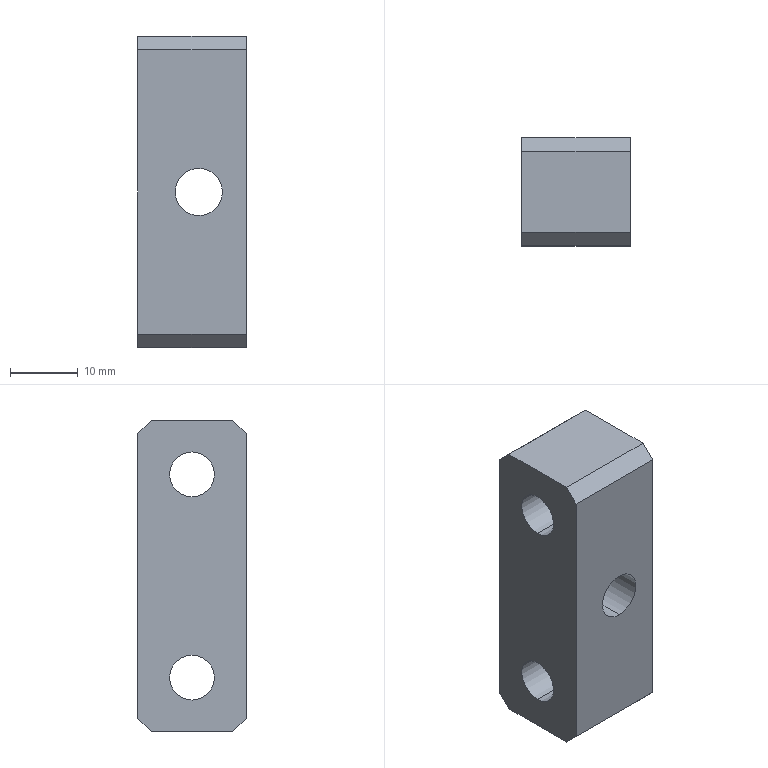Part | SolidWorks | features BaseBody 1 | 1 solid | 22 faces | box 16 x 16 x 46 mm | volume 9089 mm3 | plane 12 | cylinder 10 | commonest cylinder face diameters 6.6 x4 11 x4 6.985 x2
STEP:
#1=CARTESIAN_POINT('',(7.,0.,-20.5));
#2=VERTEX_POINT('',#1);
#3=CARTESIAN_POINT('',(7.,0.,-9.5));
#4=VERTEX_POINT('',#3);
#5=CARTESIAN_POINT('',(7.,0.,-15.));
#6=DIRECTION('',(1.,0.,0.));
#7=DIRECTION('',(0.,0.,-1.));
#8=AXIS2_PLACEMENT_3D('',#5,#6,#7);
#9=CIRCLE('',#8,5.5);
#10=EDGE_CURVE('',#2,#4,#9,.T.);
#11=ORIENTED_EDGE('',*,*,#10,.T.);
#12=CARTESIAN_POINT('',(0.,0.,-9.5));
#13=VERTEX_POINT('',#12);
#14=CARTESIAN_POINT('',(9.,0.,-9.5));
#15=DIRECTION('',(-1.,0.,0.));
#16=VECTOR('',#15,1000.);
#17=LINE('',#14,#16);
#18=EDGE_CURVE('',#4,#13,#17,.T.);
#19=ORIENTED_EDGE('',*,*,#18,.T.);
#20=CARTESIAN_POINT('',(0.,0.,-20.5));
#21=VERTEX_POINT('',#20);
#22=CARTESIAN_POINT('',(0.,0.,-15.));
#23=DIRECTION('',(1.,0.,0.));
#24=DIRECTION('',(0.,0.,-1.));
#25=AXIS2_PLACEMENT_3D('',#22,#23,#24);
#26=CIRCLE('',#25,5.5);
#27=EDGE_CURVE('',#21,#13,#26,.T.);
#28=ORIENTED_EDGE('',*,*,#27,.F.);
#29=CARTESIAN_POINT('',(9.,0.,-20.5));
#30=DIRECTION('',(-1.,0.,0.));
#31=VECTOR('',#30,1000.);
#32=LINE('',#29,#31);
#33=EDGE_CURVE('',#2,#21,#32,.T.);
#34=ORIENTED_EDGE('',*,*,#33,.F.);
#35=EDGE_LOOP('',(#11,#19,#28,#34));
#36=FACE_OUTER_BOUND('',#35,.T.);
#37=CARTESIAN_POINT('',(9.,0.,-15.));
#38=DIRECTION('',(-1.,0.,0.));
#39=DIRECTION('',(0.,0.,-1.));
#40=AXIS2_PLACEMENT_3D('',#37,#38,#39);
#41=CYLINDRICAL_SURFACE('',#40,5.5);
#42=ADVANCED_FACE('',(#36),#41,.F.);
#43=CARTESIAN_POINT('',(0.,0.,-18.3));
#44=VERTEX_POINT('',#43);
#45=CARTESIAN_POINT('',(0.,0.,-11.7));
#46=VERTEX_POINT('',#45);
#47=CARTESIAN_POINT('',(0.,0.,-15.));
#48=DIRECTION('',(1.,0.,0.));
#49=DIRECTION('',(0.,0.,-1.));
#50=AXIS2_PLACEMENT_3D('',#47,#48,#49);
#51=CIRCLE('',#50,3.3);
#52=EDGE_CURVE('',#44,#46,#51,.T.);
#53=ORIENTED_EDGE('',*,*,#52,.T.);
#54=CARTESIAN_POINT('',(-9.,0.,-11.7));
#55=VERTEX_POINT('',#54);
#56=CARTESIAN_POINT('',(-41.,0.,-11.7));
#57=DIRECTION('',(-1.,0.,0.));
#58=VECTOR('',#57,1000.);
#59=LINE('',#56,#58);
#60=EDGE_CURVE('',#46,#55,#59,.T.);
#61=ORIENTED_EDGE('',*,*,#60,.T.);
#62=CARTESIAN_POINT('',(-9.,0.,-18.3));
#63=VERTEX_POINT('',#62);
#64=CARTESIAN_POINT('',(-9.,0.,-15.));
#65=DIRECTION('',(1.,0.,0.));
#66=DIRECTION('',(0.,0.,-1.));
#67=AXIS2_PLACEMENT_3D('',#64,#65,#66);
#68=CIRCLE('',#67,3.3);
#69=EDGE_CURVE('',#63,#55,#68,.T.);
#70=ORIENTED_EDGE('',*,*,#69,.F.);
#71=CARTESIAN_POINT('',(-41.,0.,-18.3));
#72=DIRECTION('',(-1.,0.,0.));
#73=VECTOR('',#72,1000.);
#74=LINE('',#71,#73);
#75=EDGE_CURVE('',#44,#63,#74,.T.);
#76=ORIENTED_EDGE('',*,*,#75,.F.);
#77=EDGE_LOOP('',(#53,#61,#70,#76));
#78=FACE_OUTER_BOUND('',#77,.T.);
#79=CARTESIAN_POINT('',(-41.,0.,-15.));
#80=DIRECTION('',(-1.,0.,0.));
#81=DIRECTION('',(0.,0.,-1.));
#82=AXIS2_PLACEMENT_3D('',#79,#80,#81);
#83=CYLINDRICAL_SURFACE('',#82,3.3);
#84=ADVANCED_FACE('',(#78),#83,.F.);
#85=CARTESIAN_POINT('',(7.,0.,9.5));
#86=VERTEX_POINT('',#85);
#87=CARTESIAN_POINT('',(7.,0.,20.5));
#88=VERTEX_POINT('',#87);
#89=CARTESIAN_POINT('',(7.,0.,15.));
#90=DIRECTION('',(-1.,0.,0.));
#91=DIRECTION('',(0.,0.,1.));
#92=AXIS2_PLACEMENT_3D('',#89,#90,#91);
#93=CIRCLE('',#92,5.5);
#94=EDGE_CURVE('',#86,#88,#93,.T.);
#95=ORIENTED_EDGE('',*,*,#94,.F.);
#96=CARTESIAN_POINT('',(0.,0.,9.5));
#97=VERTEX_POINT('',#96);
#98=CARTESIAN_POINT('',(9.,0.,9.5));
#99=DIRECTION('',(-1.,0.,0.));
#100=VECTOR('',#99,1000.);
#101=LINE('',#98,#100);
#102=EDGE_CURVE('',#86,#97,#101,.T.);
#103=ORIENTED_EDGE('',*,*,#102,.T.);
#104=CARTESIAN_POINT('',(0.,0.,20.5));
#105=VERTEX_POINT('',#104);
#106=CARTESIAN_POINT('',(0.,0.,15.));
#107=DIRECTION('',(-1.,0.,0.));
#108=DIRECTION('',(0.,0.,1.));
#109=AXIS2_PLACEMENT_3D('',#106,#107,#108);
#110=CIRCLE('',#109,5.5);
#111=EDGE_CURVE('',#97,#105,#110,.T.);
#112=ORIENTED_EDGE('',*,*,#111,.T.);
#113=CARTESIAN_POINT('',(9.,0.,20.5));
#114=DIRECTION('',(-1.,0.,0.));
#115=VECTOR('',#114,1000.);
#116=LINE('',#113,#115);
#117=EDGE_CURVE('',#88,#105,#116,.T.);
#118=ORIENTED_EDGE('',*,*,#117,.F.);
#119=EDGE_LOOP('',(#95,#103,#112,#118));
#120=FACE_OUTER_BOUND('',#119,.T.);
#121=CARTESIAN_POINT('',(9.,0.,15.));
#122=DIRECTION('',(-1.,0.,0.));
#123=DIRECTION('',(0.,0.,1.));
#124=AXIS2_PLACEMENT_3D('',#121,#122,#123);
#125=CYLINDRICAL_SURFACE('',#124,5.5);
#126=ADVANCED_FACE('',(#120),#125,.F.);
#127=CARTESIAN_POINT('',(0.,0.,11.7));
#128=VERTEX_POINT('',#127);
#129=CARTESIAN_POINT('',(0.,0.,18.3));
#130=VERTEX_POINT('',#129);
#131=CARTESIAN_POINT('',(0.,0.,15.));
#132=DIRECTION('',(-1.,0.,0.));
#133=DIRECTION('',(0.,0.,1.));
#134=AXIS2_PLACEMENT_3D('',#131,#132,#133);
#135=CIRCLE('',#134,3.3);
#136=EDGE_CURVE('',#128,#130,#135,.T.);
#137=ORIENTED_EDGE('',*,*,#136,.F.);
#138=CARTESIAN_POINT('',(-9.,0.,11.7));
#139=VERTEX_POINT('',#138);
#140=CARTESIAN_POINT('',(-41.,0.,11.7));
#141=DIRECTION('',(-1.,0.,0.));
#142=VECTOR('',#141,1000.);
#143=LINE('',#140,#142);
#144=EDGE_CURVE('',#128,#139,#143,.T.);
#145=ORIENTED_EDGE('',*,*,#144,.T.);
#146=CARTESIAN_POINT('',(-9.,0.,18.3));
#147=VERTEX_POINT('',#146);
#148=CARTESIAN_POINT('',(-9.,0.,15.));
#149=DIRECTION('',(1.,0.,0.));
#150=DIRECTION('',(0.,0.,-1.));
#151=AXIS2_PLACEMENT_3D('',#148,#149,#150);
#152=CIRCLE('',#151,3.3);
#153=EDGE_CURVE('',#147,#139,#152,.T.);
#154=ORIENTED_EDGE('',*,*,#153,.F.);
#155=CARTESIAN_POINT('',(-41.,0.,18.3));
#156=DIRECTION('',(-1.,0.,0.));
#157=VECTOR('',#156,1000.);
#158=LINE('',#155,#157);
#159=EDGE_CURVE('',#130,#147,#158,.T.);
#160=ORIENTED_EDGE('',*,*,#159,.F.);
#161=EDGE_LOOP('',(#137,#145,#154,#160));
#162=FACE_OUTER_BOUND('',#161,.T.);
#163=CARTESIAN_POINT('',(-41.,0.,15.));
#164=DIRECTION('',(-1.,0.,0.));
#165=DIRECTION('',(0.,0.,1.));
#166=AXIS2_PLACEMENT_3D('',#163,#164,#165);
#167=CYLINDRICAL_SURFACE('',#166,3.3);
#168=ADVANCED_FACE('',(#162),#167,.F.);
#169=CARTESIAN_POINT('',(0.,-8.,-3.493));
#170=VERTEX_POINT('',#169);
#171=CARTESIAN_POINT('',(0.,-8.,3.493));
#172=VERTEX_POINT('',#171);
#173=CARTESIAN_POINT('',(0.,-8.,0.));
#174=DIRECTION('',(0.,1.,0.));
#175=DIRECTION('',(0.,0.,1.));
#176=AXIS2_PLACEMENT_3D('',#173,#174,#175);
#177=CIRCLE('',#176,3.493);
#178=EDGE_CURVE('',#170,#172,#177,.T.);
#179=ORIENTED_EDGE('',*,*,#178,.F.);
#180=CARTESIAN_POINT('',(0.,8.,-3.493));
#181=VERTEX_POINT('',#180);
#182=CARTESIAN_POINT('',(0.,-8.,-3.493));
#183=DIRECTION('',(0.,1.,0.));
#184=VECTOR('',#183,1000.);
#185=LINE('',#182,#184);
#186=EDGE_CURVE('',#170,#181,#185,.T.);
#187=ORIENTED_EDGE('',*,*,#186,.T.);
#188=CARTESIAN_POINT('',(0.,8.,3.493));
#189=VERTEX_POINT('',#188);
#190=CARTESIAN_POINT('',(0.,8.,0.));
#191=DIRECTION('',(0.,1.,0.));
#192=DIRECTION('',(0.,0.,1.));
#193=AXIS2_PLACEMENT_3D('',#190,#191,#192);
#194=CIRCLE('',#193,3.493);
#195=EDGE_CURVE('',#181,#189,#194,.T.);
#196=ORIENTED_EDGE('',*,*,#195,.T.);
#197=CARTESIAN_POINT('',(0.,-8.,3.493));
#198=DIRECTION('',(0.,1.,0.));
#199=VECTOR('',#198,1000.);
#200=LINE('',#197,#199);
#201=EDGE_CURVE('',#172,#189,#200,.T.);
#202=ORIENTED_EDGE('',*,*,#201,.F.);
#203=EDGE_LOOP('',(#179,#187,#196,#202));
#204=FACE_OUTER_BOUND('',#203,.T.);
#205=CARTESIAN_POINT('',(0.,-8.,0.));
#206=DIRECTION('',(0.,1.,0.));
#207=DIRECTION('',(0.,0.,1.));
#208=AXIS2_PLACEMENT_3D('',#205,#206,#207);
#209=CYLINDRICAL_SURFACE('',#208,3.493);
#210=ADVANCED_FACE('',(#204),#209,.F.);
#211=ORIENTED_EDGE('',*,*,#69,.T.);
#212=CARTESIAN_POINT('',(-9.,0.,-15.));
#213=DIRECTION('',(1.,0.,0.));
#214=DIRECTION('',(0.,0.,-1.));
#215=AXIS2_PLACEMENT_3D('',#212,#213,#214);
#216=CIRCLE('',#215,3.3);
#217=EDGE_CURVE('',#55,#63,#216,.T.);
#218=ORIENTED_EDGE('',*,*,#217,.T.);
#219=EDGE_LOOP('',(#211,#218));
#220=FACE_BOUND('',#219,.T.);
#221=ORIENTED_EDGE('',*,*,#153,.T.);
#222=CARTESIAN_POINT('',(-9.,0.,15.));
#223=DIRECTION('',(1.,0.,0.));
#224=DIRECTION('',(0.,0.,-1.));
#225=AXIS2_PLACEMENT_3D('',#222,#223,#224);
#226=CIRCLE('',#225,3.3);
#227=EDGE_CURVE('',#139,#147,#226,.T.);
#228=ORIENTED_EDGE('',*,*,#227,.T.);
#229=EDGE_LOOP('',(#221,#228));
#230=FACE_BOUND('',#229,.T.);
#231=CARTESIAN_POINT('',(-9.,8.,21.));
#232=VERTEX_POINT('',#231);
#233=CARTESIAN_POINT('',(-9.,8.,-21.));
#234=VERTEX_POINT('',#233);
#235=CARTESIAN_POINT('',(-9.,8.,23.));
#236=DIRECTION('',(0.,0.,-1.));
#237=VECTOR('',#236,1000.);
#238=LINE('',#235,#237);
#239=EDGE_CURVE('',#232,#234,#238,.T.);
#240=ORIENTED_EDGE('',*,*,#239,.T.);
#241=CARTESIAN_POINT('',(-9.,6.,-23.));
#242=VERTEX_POINT('',#241);
#243=CARTESIAN_POINT('',(-9.,6.,-23.));
#244=DIRECTION('',(0.,-0.7071,-0.7071));
#245=VECTOR('',#244,1000.);
#246=LINE('',#243,#245);
#247=EDGE_CURVE('',#234,#242,#246,.T.);
#248=ORIENTED_EDGE('',*,*,#247,.T.);
#249=CARTESIAN_POINT('',(-9.,-6.,-23.));
#250=VERTEX_POINT('',#249);
#251=CARTESIAN_POINT('',(-9.,-8.,-23.));
#252=DIRECTION('',(0.,1.,0.));
#253=VECTOR('',#252,1000.);
#254=LINE('',#251,#253);
#255=EDGE_CURVE('',#250,#242,#254,.T.);
#256=ORIENTED_EDGE('',*,*,#255,.F.);
#257=CARTESIAN_POINT('',(-9.,-8.,-21.));
#258=VERTEX_POINT('',#257);
#259=CARTESIAN_POINT('',(-9.,-8.,-21.));
#260=DIRECTION('',(0.,-0.7071,0.7071));
#261=VECTOR('',#260,1000.);
#262=LINE('',#259,#261);
#263=EDGE_CURVE('',#250,#258,#262,.T.);
#264=ORIENTED_EDGE('',*,*,#263,.T.);
#265=CARTESIAN_POINT('',(-9.,-8.,21.));
#266=VERTEX_POINT('',#265);
#267=CARTESIAN_POINT('',(-9.,-8.,23.));
#268=DIRECTION('',(0.,0.,-1.));
#269=VECTOR('',#268,1000.);
#270=LINE('',#267,#269);
#271=EDGE_CURVE('',#266,#258,#270,.T.);
#272=ORIENTED_EDGE('',*,*,#271,.F.);
#273=CARTESIAN_POINT('',(-9.,-6.,23.));
#274=VERTEX_POINT('',#273);
#275=CARTESIAN_POINT('',(-9.,-8.,21.));
#276=DIRECTION('',(0.,0.7071,0.7071));
#277=VECTOR('',#276,1000.);
#278=LINE('',#275,#277);
#279=EDGE_CURVE('',#266,#274,#278,.T.);
#280=ORIENTED_EDGE('',*,*,#279,.T.);
#281=CARTESIAN_POINT('',(-9.,6.,23.));
#282=VERTEX_POINT('',#281);
#283=CARTESIAN_POINT('',(-9.,-8.,23.));
#284=DIRECTION('',(0.,1.,0.));
#285=VECTOR('',#284,1000.);
#286=LINE('',#283,#285);
#287=EDGE_CURVE('',#274,#282,#286,.T.);
#288=ORIENTED_EDGE('',*,*,#287,.T.);
#289=CARTESIAN_POINT('',(-9.,6.,23.));
#290=DIRECTION('',(0.,0.7071,-0.7071));
#291=VECTOR('',#290,1000.);
#292=LINE('',#289,#291);
#293=EDGE_CURVE('',#282,#232,#292,.T.);
#294=ORIENTED_EDGE('',*,*,#293,.T.);
#295=EDGE_LOOP('',(#240,#248,#256,#264,#272,#280,#288,#294));
#296=FACE_OUTER_BOUND('',#295,.T.);
#297=CARTESIAN_POINT('',(-9.,-8.,23.));
#298=DIRECTION('',(1.,0.,0.));
#299=DIRECTION('',(0.,0.,-1.));
#300=AXIS2_PLACEMENT_3D('',#297,#298,#299);
#301=PLANE('',#300);
#302=ADVANCED_FACE('',(#220,#230,#296),#301,.F.);
#303=ORIENTED_EDGE('',*,*,#255,.T.);
#304=CARTESIAN_POINT('',(7.,6.,-23.));
#305=VERTEX_POINT('',#304);
#306=CARTESIAN_POINT('',(9.,6.,-23.));
#307=DIRECTION('',(1.,0.,0.));
#308=VECTOR('',#307,1000.);
#309=LINE('',#306,#308);
#310=EDGE_CURVE('',#242,#305,#309,.T.);
#311=ORIENTED_EDGE('',*,*,#310,.T.);
#312=CARTESIAN_POINT('',(7.,-6.,-23.));
#313=VERTEX_POINT('',#312);
#314=CARTESIAN_POINT('',(7.,-8.,-23.));
#315=DIRECTION('',(0.,1.,0.));
#316=VECTOR('',#315,1000.);
#317=LINE('',#314,#316);
#318=EDGE_CURVE('',#313,#305,#317,.T.);
#319=ORIENTED_EDGE('',*,*,#318,.F.);
#320=CARTESIAN_POINT('',(-9.,-6.,-23.));
#321=DIRECTION('',(-1.,0.,0.));
#322=VECTOR('',#321,1000.);
#323=LINE('',#320,#322);
#324=EDGE_CURVE('',#313,#250,#323,.T.);
#325=ORIENTED_EDGE('',*,*,#324,.T.);
#326=EDGE_LOOP('',(#303,#311,#319,#325));
#327=FACE_OUTER_BOUND('',#326,.T.);
#328=CARTESIAN_POINT('',(-9.,-8.,-23.));
#329=DIRECTION('',(0.,0.,1.));
#330=DIRECTION('',(1.,0.,0.));
#331=AXIS2_PLACEMENT_3D('',#328,#329,#330);
#332=PLANE('',#331);
#333=ADVANCED_FACE('',(#327),#332,.F.);
#334=ORIENTED_EDGE('',*,*,#10,.F.);
#335=CARTESIAN_POINT('',(7.,0.,-15.));
#336=DIRECTION('',(1.,0.,0.));
#337=DIRECTION('',(0.,0.,-1.));
#338=AXIS2_PLACEMENT_3D('',#335,#336,#337);
#339=CIRCLE('',#338,5.5);
#340=EDGE_CURVE('',#4,#2,#339,.T.);
#341=ORIENTED_EDGE('',*,*,#340,.F.);
#342=EDGE_LOOP('',(#334,#341));
#343=FACE_BOUND('',#342,.T.);
#344=CARTESIAN_POINT('',(7.,0.,15.));
#345=DIRECTION('',(-1.,0.,0.));
#346=DIRECTION('',(0.,0.,1.));
#347=AXIS2_PLACEMENT_3D('',#344,#345,#346);
#348=CIRCLE('',#347,5.5);
#349=EDGE_CURVE('',#88,#86,#348,.T.);
#350=ORIENTED_EDGE('',*,*,#349,.T.);
#351=ORIENTED_EDGE('',*,*,#94,.T.);
#352=EDGE_LOOP('',(#350,#351));
#353=FACE_BOUND('',#352,.T.);
#354=ORIENTED_EDGE('',*,*,#318,.T.);
#355=CARTESIAN_POINT('',(7.,8.,-21.));
#356=VERTEX_POINT('',#355);
#357=CARTESIAN_POINT('',(7.,6.,-23.));
#358=DIRECTION('',(0.,0.7071,0.7071));
#359=VECTOR('',#358,1000.);
#360=LINE('',#357,#359);
#361=EDGE_CURVE('',#305,#356,#360,.T.);
#362=ORIENTED_EDGE('',*,*,#361,.T.);
#363=CARTESIAN_POINT('',(7.,8.,21.));
#364=VERTEX_POINT('',#363);
#365=CARTESIAN_POINT('',(7.,8.,-23.));
#366=DIRECTION('',(0.,0.,1.));
#367=VECTOR('',#366,1000.);
#368=LINE('',#365,#367);
#369=EDGE_CURVE('',#356,#364,#368,.T.);
#370=ORIENTED_EDGE('',*,*,#369,.T.);
#371=CARTESIAN_POINT('',(7.,6.,23.));
#372=VERTEX_POINT('',#371);
#373=CARTESIAN_POINT('',(7.,6.,23.));
#374=DIRECTION('',(0.,-0.7071,0.7071));
#375=VECTOR('',#374,1000.);
#376=LINE('',#373,#375);
#377=EDGE_CURVE('',#364,#372,#376,.T.);
#378=ORIENTED_EDGE('',*,*,#377,.T.);
#379=CARTESIAN_POINT('',(7.,-6.,23.));
#380=VERTEX_POINT('',#379);
#381=CARTESIAN_POINT('',(7.,-8.,23.));
#382=DIRECTION('',(0.,1.,0.));
#383=VECTOR('',#382,1000.);
#384=LINE('',#381,#383);
#385=EDGE_CURVE('',#380,#372,#384,.T.);
#386=ORIENTED_EDGE('',*,*,#385,.F.);
#387=CARTESIAN_POINT('',(7.,-8.,21.));
#388=VERTEX_POINT('',#387);
#389=CARTESIAN_POINT('',(7.,-8.,21.));
#390=DIRECTION('',(0.,-0.7071,-0.7071));
#391=VECTOR('',#390,1000.);
#392=LINE('',#389,#391);
#393=EDGE_CURVE('',#380,#388,#392,.T.);
#394=ORIENTED_EDGE('',*,*,#393,.T.);
#395=CARTESIAN_POINT('',(7.,-8.,-21.));
#396=VERTEX_POINT('',#395);
#397=CARTESIAN_POINT('',(7.,-8.,-23.));
#398=DIRECTION('',(0.,0.,1.));
#399=VECTOR('',#398,1000.);
#400=LINE('',#397,#399);
#401=EDGE_CURVE('',#396,#388,#400,.T.);
#402=ORIENTED_EDGE('',*,*,#401,.F.);
#403=CARTESIAN_POINT('',(7.,-8.,-21.));
#404=DIRECTION('',(0.,0.7071,-0.7071));
#405=VECTOR('',#404,1000.);
#406=LINE('',#403,#405);
#407=EDGE_CURVE('',#396,#313,#406,.T.);
#408=ORIENTED_EDGE('',*,*,#407,.T.);
#409=EDGE_LOOP('',(#354,#362,#370,#378,#386,#394,#402,#408));
#410=FACE_OUTER_BOUND('',#409,.T.);
#411=CARTESIAN_POINT('',(7.,-8.,-23.));
#412=DIRECTION('',(-1.,0.,0.));
#413=DIRECTION('',(0.,0.,1.));
#414=AXIS2_PLACEMENT_3D('',#411,#412,#413);
#415=PLANE('',#414);
#416=ADVANCED_FACE('',(#343,#353,#410),#415,.F.);
#417=ORIENTED_EDGE('',*,*,#385,.T.);
#418=CARTESIAN_POINT('',(-9.,6.,23.));
#419=DIRECTION('',(-1.,0.,0.));
#420=VECTOR('',#419,1000.);
#421=LINE('',#418,#420);
#422=EDGE_CURVE('',#372,#282,#421,.T.);
#423=ORIENTED_EDGE('',*,*,#422,.T.);
#424=ORIENTED_EDGE('',*,*,#287,.F.);
#425=CARTESIAN_POINT('',(9.,-6.,23.));
#426=DIRECTION('',(1.,0.,0.));
#427=VECTOR('',#426,1000.);
#428=LINE('',#425,#427);
#429=EDGE_CURVE('',#274,#380,#428,.T.);
#430=ORIENTED_EDGE('',*,*,#429,.T.);
#431=EDGE_LOOP('',(#417,#423,#424,#430));
#432=FACE_OUTER_BOUND('',#431,.T.);
#433=CARTESIAN_POINT('',(9.,-8.,23.));
#434=DIRECTION('',(0.,0.,-1.));
#435=DIRECTION('',(-1.,0.,0.));
#436=AXIS2_PLACEMENT_3D('',#433,#434,#435);
#437=PLANE('',#436);
#438=ADVANCED_FACE('',(#432),#437,.F.);
#439=CARTESIAN_POINT('',(0.,-8.,0.));
#440=DIRECTION('',(0.,1.,0.));
#441=DIRECTION('',(0.,0.,1.));
#442=AXIS2_PLACEMENT_3D('',#439,#440,#441);
#443=CIRCLE('',#442,3.493);
#444=EDGE_CURVE('',#172,#170,#443,.T.);
#445=ORIENTED_EDGE('',*,*,#444,.T.);
#446=ORIENTED_EDGE('',*,*,#178,.T.);
#447=EDGE_LOOP('',(#445,#446));
#448=FACE_BOUND('',#447,.T.);
#449=ORIENTED_EDGE('',*,*,#271,.T.);
#450=CARTESIAN_POINT('',(-9.,-8.,-21.));
#451=DIRECTION('',(1.,0.,0.));
#452=VECTOR('',#451,1000.);
#453=LINE('',#450,#452);
#454=EDGE_CURVE('',#258,#396,#453,.T.);
#455=ORIENTED_EDGE('',*,*,#454,.T.);
#456=ORIENTED_EDGE('',*,*,#401,.T.);
#457=CARTESIAN_POINT('',(-9.,-8.,21.));
#458=DIRECTION('',(-1.,0.,0.));
#459=VECTOR('',#458,1000.);
#460=LINE('',#457,#459);
#461=EDGE_CURVE('',#388,#266,#460,.T.);
#462=ORIENTED_EDGE('',*,*,#461,.T.);
#463=EDGE_LOOP('',(#449,#455,#456,#462));
#464=FACE_OUTER_BOUND('',#463,.T.);
#465=CARTESIAN_POINT('',(-9.,-8.,23.));
#466=DIRECTION('',(0.,1.,0.));
#467=DIRECTION('',(0.,0.,1.));
#468=AXIS2_PLACEMENT_3D('',#465,#466,#467);
#469=PLANE('',#468);
#470=ADVANCED_FACE('',(#448,#464),#469,.F.);
#471=CARTESIAN_POINT('',(0.,8.,0.));
#472=DIRECTION('',(0.,1.,0.));
#473=DIRECTION('',(0.,0.,1.));
#474=AXIS2_PLACEMENT_3D('',#471,#472,#473);
#475=CIRCLE('',#474,3.493);
#476=EDGE_CURVE('',#189,#181,#475,.T.);
#477=ORIENTED_EDGE('',*,*,#476,.F.);
#478=ORIENTED_EDGE('',*,*,#195,.F.);
#479=EDGE_LOOP('',(#477,#478));
#480=FACE_BOUND('',#479,.T.);
#481=ORIENTED_EDGE('',*,*,#369,.F.);
#482=CARTESIAN_POINT('',(-9.,8.,-21.));
#483=DIRECTION('',(-1.,0.,0.));
#484=VECTOR('',#483,1000.);
#485=LINE('',#482,#484);
#486=EDGE_CURVE('',#356,#234,#485,.T.);
#487=ORIENTED_EDGE('',*,*,#486,.T.);
#488=ORIENTED_EDGE('',*,*,#239,.F.);
#489=CARTESIAN_POINT('',(9.,8.,21.));
#490=DIRECTION('',(1.,0.,0.));
#491=VECTOR('',#490,1000.);
#492=LINE('',#489,#491);
#493=EDGE_CURVE('',#232,#364,#492,.T.);
#494=ORIENTED_EDGE('',*,*,#493,.T.);
#495=EDGE_LOOP('',(#481,#487,#488,#494));
#496=FACE_OUTER_BOUND('',#495,.T.);
#497=CARTESIAN_POINT('',(-9.,8.,23.));
#498=DIRECTION('',(0.,1.,0.));
#499=DIRECTION('',(0.,0.,1.));
#500=AXIS2_PLACEMENT_3D('',#497,#498,#499);
#501=PLANE('',#500);
#502=ADVANCED_FACE('',(#480,#496),#501,.T.);
#503=ORIENTED_EDGE('',*,*,#186,.F.);
#504=ORIENTED_EDGE('',*,*,#444,.F.);
#505=ORIENTED_EDGE('',*,*,#201,.T.);
#506=ORIENTED_EDGE('',*,*,#476,.T.);
#507=EDGE_LOOP('',(#503,#504,#505,#506));
#508=FACE_OUTER_BOUND('',#507,.T.);
#509=CARTESIAN_POINT('',(0.,-8.,0.));
#510=DIRECTION('',(0.,1.,0.));
#511=DIRECTION('',(0.,0.,1.));
#512=AXIS2_PLACEMENT_3D('',#509,#510,#511);
#513=CYLINDRICAL_SURFACE('',#512,3.493);
#514=ADVANCED_FACE('',(#508),#513,.F.);
#515=ORIENTED_EDGE('',*,*,#144,.F.);
#516=CARTESIAN_POINT('',(0.,0.,15.));
#517=DIRECTION('',(-1.,0.,0.));
#518=DIRECTION('',(0.,0.,1.));
#519=AXIS2_PLACEMENT_3D('',#516,#517,#518);
#520=CIRCLE('',#519,3.3);
#521=EDGE_CURVE('',#130,#128,#520,.T.);
#522=ORIENTED_EDGE('',*,*,#521,.F.);
#523=ORIENTED_EDGE('',*,*,#159,.T.);
#524=ORIENTED_EDGE('',*,*,#227,.F.);
#525=EDGE_LOOP('',(#515,#522,#523,#524));
#526=FACE_OUTER_BOUND('',#525,.T.);
#527=CARTESIAN_POINT('',(-41.,0.,15.));
#528=DIRECTION('',(-1.,0.,0.));
#529=DIRECTION('',(0.,0.,1.));
#530=AXIS2_PLACEMENT_3D('',#527,#528,#529);
#531=CYLINDRICAL_SURFACE('',#530,3.3);
#532=ADVANCED_FACE('',(#526),#531,.F.);
#533=ORIENTED_EDGE('',*,*,#521,.T.);
#534=ORIENTED_EDGE('',*,*,#136,.T.);
#535=EDGE_LOOP('',(#533,#534));
#536=FACE_BOUND('',#535,.T.);
#537=CARTESIAN_POINT('',(0.,0.,15.));
#538=DIRECTION('',(-1.,0.,0.));
#539=DIRECTION('',(0.,0.,1.));
#540=AXIS2_PLACEMENT_3D('',#537,#538,#539);
#541=CIRCLE('',#540,5.5);
#542=EDGE_CURVE('',#105,#97,#541,.T.);
#543=ORIENTED_EDGE('',*,*,#542,.F.);
#544=ORIENTED_EDGE('',*,*,#111,.F.);
#545=EDGE_LOOP('',(#543,#544));
#546=FACE_OUTER_BOUND('',#545,.T.);
#547=CARTESIAN_POINT('',(0.,0.,15.));
#548=DIRECTION('',(-1.,0.,0.));
#549=DIRECTION('',(0.,0.,1.));
#550=AXIS2_PLACEMENT_3D('',#547,#548,#549);
#551=PLANE('',#550);
#552=ADVANCED_FACE('',(#536,#546),#551,.F.);
#553=ORIENTED_EDGE('',*,*,#102,.F.);
#554=ORIENTED_EDGE('',*,*,#349,.F.);
#555=ORIENTED_EDGE('',*,*,#117,.T.);
#556=ORIENTED_EDGE('',*,*,#542,.T.);
#557=EDGE_LOOP('',(#553,#554,#555,#556));
#558=FACE_OUTER_BOUND('',#557,.T.);
#559=CARTESIAN_POINT('',(9.,0.,15.));
#560=DIRECTION('',(-1.,0.,0.));
#561=DIRECTION('',(0.,0.,1.));
#562=AXIS2_PLACEMENT_3D('',#559,#560,#561);
#563=CYLINDRICAL_SURFACE('',#562,5.5);
#564=ADVANCED_FACE('',(#558),#563,.F.);
#565=ORIENTED_EDGE('',*,*,#60,.F.);
#566=CARTESIAN_POINT('',(0.,0.,-15.));
#567=DIRECTION('',(1.,0.,0.));
#568=DIRECTION('',(0.,0.,-1.));
#569=AXIS2_PLACEMENT_3D('',#566,#567,#568);
#570=CIRCLE('',#569,3.3);
#571=EDGE_CURVE('',#46,#44,#570,.T.);
#572=ORIENTED_EDGE('',*,*,#571,.T.);
#573=ORIENTED_EDGE('',*,*,#75,.T.);
#574=ORIENTED_EDGE('',*,*,#217,.F.);
#575=EDGE_LOOP('',(#565,#572,#573,#574));
#576=FACE_OUTER_BOUND('',#575,.T.);
#577=CARTESIAN_POINT('',(-41.,0.,-15.));
#578=DIRECTION('',(-1.,0.,0.));
#579=DIRECTION('',(0.,0.,-1.));
#580=AXIS2_PLACEMENT_3D('',#577,#578,#579);
#581=CYLINDRICAL_SURFACE('',#580,3.3);
#582=ADVANCED_FACE('',(#576),#581,.F.);
#583=ORIENTED_EDGE('',*,*,#52,.F.);
#584=ORIENTED_EDGE('',*,*,#571,.F.);
#585=EDGE_LOOP('',(#583,#584));
#586=FACE_BOUND('',#585,.T.);
#587=ORIENTED_EDGE('',*,*,#27,.T.);
#588=CARTESIAN_POINT('',(0.,0.,-15.));
#589=DIRECTION('',(1.,0.,0.));
#590=DIRECTION('',(0.,0.,-1.));
#591=AXIS2_PLACEMENT_3D('',#588,#589,#590);
#592=CIRCLE('',#591,5.5);
#593=EDGE_CURVE('',#13,#21,#592,.T.);
#594=ORIENTED_EDGE('',*,*,#593,.T.);
#595=EDGE_LOOP('',(#587,#594));
#596=FACE_OUTER_BOUND('',#595,.T.);
#597=CARTESIAN_POINT('',(0.,0.,-15.));
#598=DIRECTION('',(-1.,0.,0.));
#599=DIRECTION('',(0.,0.,-1.));
#600=AXIS2_PLACEMENT_3D('',#597,#598,#599);
#601=PLANE('',#600);
#602=ADVANCED_FACE('',(#586,#596),#601,.F.);
#603=ORIENTED_EDGE('',*,*,#18,.F.);
#604=ORIENTED_EDGE('',*,*,#340,.T.);
#605=ORIENTED_EDGE('',*,*,#33,.T.);
#606=ORIENTED_EDGE('',*,*,#593,.F.);
#607=EDGE_LOOP('',(#603,#604,#605,#606));
#608=FACE_OUTER_BOUND('',#607,.T.);
#609=CARTESIAN_POINT('',(9.,0.,-15.));
#610=DIRECTION('',(-1.,0.,0.));
#611=DIRECTION('',(0.,0.,-1.));
#612=AXIS2_PLACEMENT_3D('',#609,#610,#611);
#613=CYLINDRICAL_SURFACE('',#612,5.5);
#614=ADVANCED_FACE('',(#608),#613,.F.);
#615=ORIENTED_EDGE('',*,*,#247,.F.);
#616=ORIENTED_EDGE('',*,*,#486,.F.);
#617=ORIENTED_EDGE('',*,*,#361,.F.);
#618=ORIENTED_EDGE('',*,*,#310,.F.);
#619=EDGE_LOOP('',(#615,#616,#617,#618));
#620=FACE_OUTER_BOUND('',#619,.T.);
#621=CARTESIAN_POINT('',(-9.,6.,-23.));
#622=DIRECTION('',(0.,0.7071,-0.7071));
#623=DIRECTION('',(0.,0.7071,0.7071));
#624=AXIS2_PLACEMENT_3D('',#621,#622,#623);
#625=PLANE('',#624);
#626=ADVANCED_FACE('',(#620),#625,.T.);
#627=ORIENTED_EDGE('',*,*,#263,.F.);
#628=ORIENTED_EDGE('',*,*,#324,.F.);
#629=ORIENTED_EDGE('',*,*,#407,.F.);
#630=ORIENTED_EDGE('',*,*,#454,.F.);
#631=EDGE_LOOP('',(#627,#628,#629,#630));
#632=FACE_OUTER_BOUND('',#631,.T.);
#633=CARTESIAN_POINT('',(-9.,-8.,-21.));
#634=DIRECTION('',(0.,0.7071,0.7071));
#635=DIRECTION('',(0.,-0.7071,0.7071));
#636=AXIS2_PLACEMENT_3D('',#633,#634,#635);
#637=PLANE('',#636);
#638=ADVANCED_FACE('',(#632),#637,.F.);
#639=ORIENTED_EDGE('',*,*,#377,.F.);
#640=ORIENTED_EDGE('',*,*,#493,.F.);
#641=ORIENTED_EDGE('',*,*,#293,.F.);
#642=ORIENTED_EDGE('',*,*,#422,.F.);
#643=EDGE_LOOP('',(#639,#640,#641,#642));
#644=FACE_OUTER_BOUND('',#643,.T.);
#645=CARTESIAN_POINT('',(9.,6.,23.));
#646=DIRECTION('',(0.,0.7071,0.7071));
#647=DIRECTION('',(0.,-0.7071,0.7071));
#648=AXIS2_PLACEMENT_3D('',#645,#646,#647);
#649=PLANE('',#648);
#650=ADVANCED_FACE('',(#644),#649,.T.);
#651=ORIENTED_EDGE('',*,*,#393,.F.);
#652=ORIENTED_EDGE('',*,*,#429,.F.);
#653=ORIENTED_EDGE('',*,*,#279,.F.);
#654=ORIENTED_EDGE('',*,*,#461,.F.);
#655=EDGE_LOOP('',(#651,#652,#653,#654));
#656=FACE_OUTER_BOUND('',#655,.T.);
#657=CARTESIAN_POINT('',(-9.,-8.,21.));
#658=DIRECTION('',(0.,0.7071,-0.7071));
#659=DIRECTION('',(0.,0.7071,0.7071));
#660=AXIS2_PLACEMENT_3D('',#657,#658,#659);
#661=PLANE('',#660);
#662=ADVANCED_FACE('',(#656),#661,.F.);
#663=CLOSED_SHELL('',(#42,#84,#126,#168,#210,#302,#333,#416,#438,#470,#502,#514,#532,#552,#564,#582,#602,#614,#626,#638,#650,#662));
#664=MANIFOLD_SOLID_BREP('',#663);
#665=CARTESIAN_POINT('',(0.,0.,0.));
#666=DIRECTION('',(0.,0.,1.));
#667=DIRECTION('',(1.,0.,0.));
#668=AXIS2_PLACEMENT_3D('',#665,#666,#667);
#669=(LENGTH_UNIT()NAMED_UNIT(*)SI_UNIT(.MILLI.,.METRE.));
#670=UNCERTAINTY_MEASURE_WITH_UNIT(LENGTH_MEASURE(0.00001),#669,'','');
#671=(NAMED_UNIT(*)PLANE_ANGLE_UNIT()SI_UNIT($,.RADIAN.));
#672=(NAMED_UNIT(*)SI_UNIT($,.STERADIAN.)SOLID_ANGLE_UNIT());
#673=(GEOMETRIC_REPRESENTATION_CONTEXT(3)GLOBAL_UNCERTAINTY_ASSIGNED_CONTEXT((#670))GLOBAL_UNIT_ASSIGNED_CONTEXT((#669,#671,#672))REPRESENTATION_CONTEXT('',''));
#674=ADVANCED_BREP_SHAPE_REPRESENTATION('',(#664,#668),#673);